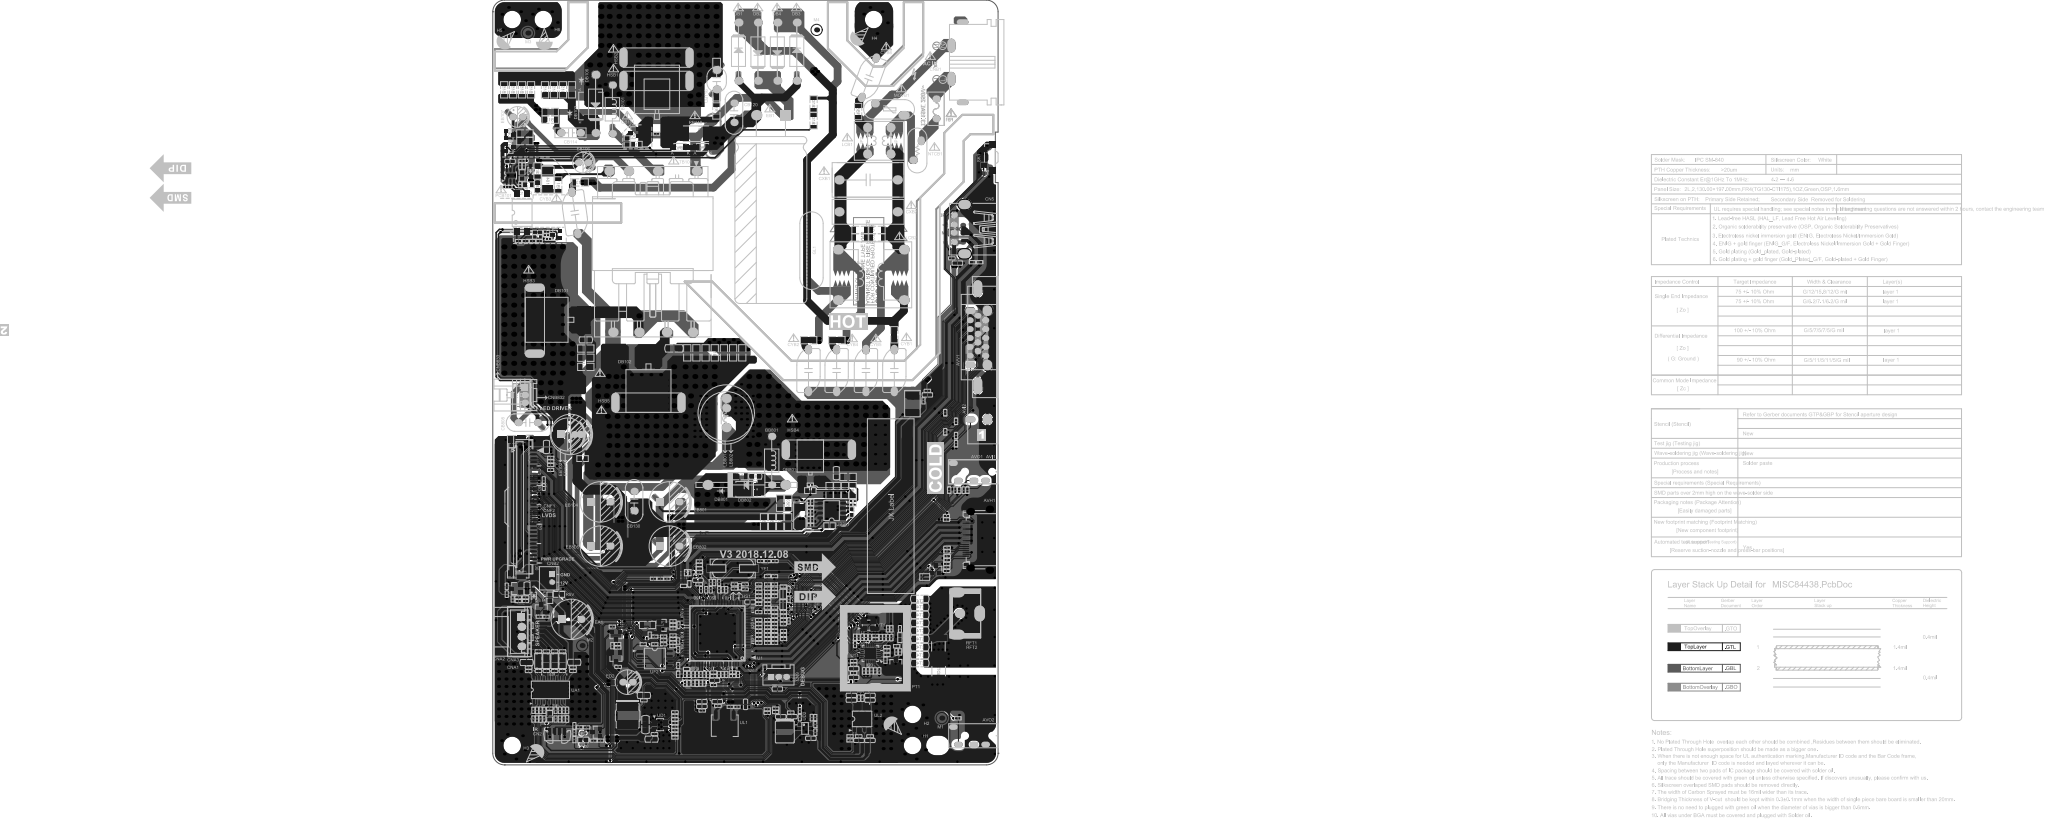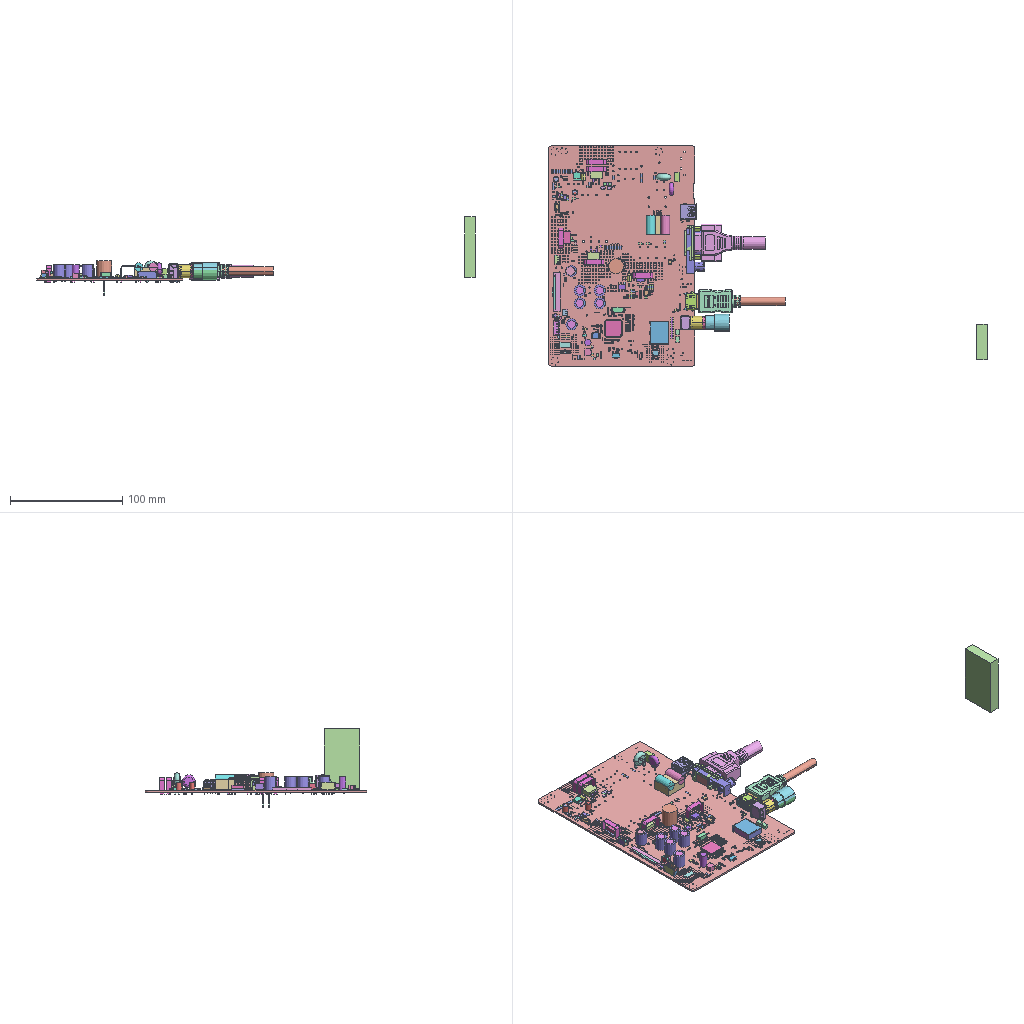Circuit board layout | Altium Designer | box 390.7 x 197 x 69.7 mm
Layer stack:
# Altium Designer layer stack of  (unit mm; dielectric type: 0 none, 1 core, 2 prepreg, 3 surface material)
index,name,kind,layer,copper_thickness_mm,dielectric_type,dielectric_thickness_mm,dielectric_material,dielectric_constant
0,TopPaste,other,,,,,,
1,TopOverlay,other,,,,,,
2,TopSolder,dielectric,,,3,0.0102,Solder Resist,3.5
3,TopLayer,copper,TopLayer,0.0356,,,,
4,Dielectric1,dielectric,,,1,1.5,FR-4,4.8
5,BottomLayer,copper,BottomLayer,0.0356,,,,
6,BottomSolder,dielectric,,,3,0.0102,Solder Resist,3.5
7,BottomOverlay,other,,,,,,
8,BottomPaste,other,,,,,,
# drill layer pairs: low layer,high layer
drill_pair,TopLayer,BottomLayer
Part placement, first 381 of 575 lines:
Designator,Comment,Layer,Footprint,Center-X(mm),Center-Y(mm),Rotation
CYB6,Y capacitor,CAP Y1,CD,100pF,400VAC,±10%,KS,10mm,Y5P,DIP,Walsin,TopLayer,CAP13*5-V-10-1,-33.2,177,70
CB116,Ceramic capacitor,CAP CD,2KV,68pF,±5%,SL,IK,5.0mm,DIP,TP,Walsin,TopLayer,CAP6.5*5-V-5-1,-72.401,176.521,90
CB120,Ceramic capacitor,CAP CD,2KV,4700pF,±20%,Y5U,IK,5.0mm,DIP,TP,Walsin,TopLayer,CAP10*4.5-V-5,-67.939,167.989,90
RB119,Thick-film resistor,RES,1/4W,10ohm,±5%,1206,SMD,TopLayer,R1206,-72.477,168.453,90
CNF1,NC/FFC socket,FFC connector,30Pin,D1.0,Bottom,lock,SMD,F10033FA030M1WL,CT,TopLayer,FFC30H/1.0S-7,-122.333,66.5,270
CAUTION,CAUTION,BottomLayer,CAUTION,-684.727,-474.313,90
TB-GND2,NC/TEST,BottomLayer,TP-10,-35.979,193.624,90
TB-GND1,NC/TEST,BottomLayer,TP-10,-119.545,188.239,90
H6,Location hole,TopLayer,ASSE4.0C-3,-116.613,191.96,0
H5,Location hole,TopLayer,ASSE4.0C-3,-124.715,191.746,0
HOT,HOT,TopLayer,HOT,-684.727,-474.313,360
High Voltage,High Voltage,TopLayer,High_Voltage,-684.727,-474.313,360
H4,Location hole,TopLayer,ASSE4.0C-3,-31.653,191.758,0
COLD,COLD,TopLayer,COLD,-684.727,-474.313,90
M3,MARK,TopLayer,MARK,-120.968,188.519,0
M4,MARK,TopLayer,MARK,-46.685,189.332,0
RB106,Thick-film resistor,RES,1/8W,68ohm,±5%,0805,SMD,TopLayer,R0805,-93.04,159.88,360
CB801,Ceramic capacitor,CAP MC,25V,1uF,±10%,X7R,0603,SMD,TP,TopLayer,C0603,-37.668,65.113,270
RB816,10ohm-0805-±5%-1/8W,TopLayer,R0805,-43.355,61.595,360
BB101,Ferrite bead,BEAD,70ohmMin,f3.5×6.0×0.65,DIP,TP,RH3.5×6×0.8-T-LF,DL,TopLayer,LB/3.5*6*12.5,-99.228,168.874,270
DB106,Rectifier diode,DIO FRD S,2A,1000V,DO-15,DIP,FR207G-FG-WS,WILLAS,TopLayer,D2-H-15,-103.554,170.282,270
CXB1,X capacitor,CAP X2,MP,275VAC,0.47uF,±10%,S,15mm-Mini,PC,DIP,BM,TopLayer,CAP18*8.5-V-15,-33.432,150.692,180
JP2,NC/Jumper,RES JUMP,0.6,7.0mm,DIP,TopLayer,JP7.0,-33.582,160.763,90
JP1,NC/Jumper,RES JUMP,0.6,7.0mm,DIP,TopLayer,JP7.0,-27.582,160.763,90
NTCB1,SCK102R55AMBY502 (short leg / Weiqin),TopLayer,NTC(10*5)-V5,-20.812,158.268,90
TB101,Transformer,EQ2914,310uH,0.30×2P,29Ts,H14.5MAX,SYEQ2914Z-T012021A (BLACK),DIP,YX,TopLayer,T/EQ2914*9-1,-88.835,132.192,270
LB802,NC/Differential-mode inductor,Inductor,DR12×14,68uH,0.45,20Ts,H13.5MAX,SYDR1214-L068uA,DIP,Soldier,TopLayer,L(13.5*15.5)-V-5,-69.945,89.4,90
RB835,Thick-film resistor,RES,1/4W,270Kohm,±1%,1206-Auto,SMD,TopLayer,R1206,-53.993,67.399,90
LCB2,Common-mode choke,Common Choke,UC1614,10.5mH±10%,0.15×1.0mm,48Ts,H14.0MAX,SYUC16-L10.5mA,DIP,CH,TopLayer,L/LC4/21*17-H-17*13,-32.722,126.231,180
BB801,Ferrite bead,BEAD,30ohmMin,F3.5×3.0×0.65,DIP,TP,RH3.5×3×0.8-T-LF,DL,TopLayer,LB/3.5*6*12.5,-58.242,78.364,270
CB101,100pF-0402-NPO-±5%-50V,TopLayer,C0402,-122.936,154.254,270
CB102,0.1uF-0603-X7R-±10%-50V,TopLayer,C0603,-125.565,155.473,180
CB103,Ceramic capacitor,CAP MC,50V,1000pF,±20%,X7R,0402,SMD,TP,TopLayer,C0402,-125.882,148.882,180
CB109,Ceramic capacitor,CAP MC,25V,0.22uF,±10%,X7R,0603,SMD,TP,TopLayer,C0603,-118.504,137.198,360
CB110,NC/1000pF-0402-X7R-±10%-50V,TopLayer,C0402,-116.205,137.351,360
CB113,NC/220PF-0805-NPO-±10%-200V,TopLayer,C0805,-118.478,149.022,90
CB114,Film capacitor,CAP PE,400V,4700pF,±5%,P,5.0mm,PC,DIP,TP,Fara,TopLayer,CAP8*2.5-V-5,-110.007,162.814,360
CB117,1000pF-0805-NPO-±10%-200V,TopLayer,C0805,-106.07,109.479,360
CB118,Ceramic capacitor,CAP MC,1KV,1000pF,±5%,NPO,1206,SMD,TP,TopLayer,C1206,-83.384,107.288,360
CB125,NC/Ceramic capacitor,CAP MC,50V,0.022uF,±10%,X7R,0402,SMD,TP,TopLayer,C0402,-121.59,134.925,360
CB130,Ceramic capacitor,CAP CD,1KV,4700pF,±20%,Y5U,IK,5.0mm,DIP,TP,Walsin,TopLayer,CAP10*4.5-V-5,-93.638,67.958,90
CB803,100pF-0402-NPO-±5%-50V,TopLayer,C0402,-37.821,67.496,90
CB804,4700pF-0402-X7R-±10%-50V,TopLayer,C0402,-47.803,67.653,90
CB805,NC/0.1uF-0402-X7R-±10%-16V,TopLayer,C0402,-48.73,64.91,90
CB806,Ceramic capacitor,CAP MC,50V,1000pF,±20%,X7R,0402,SMD,TP,TopLayer,C0402,-47.803,63.132,270
CB808,NC/Ceramic capacitor,CAP CD,1KV,4700pF,±20%,Y5U,K,5.0mm,DIP,TP,Walsin,TopLayer,CAP10*4.5-V-5,-120.983,88.168,180
CB809,Ceramic capacitor,CAP MC,500V,220pF,±5%,NPO,0805,SMD,TP,TopLayer,C0805,-41.618,75.146,90
CB810,Ceramic capacitor,CAP MC,500V,220pF,±5%,NPO,0805,SMD,TP,TopLayer,C0805,-62.466,74.364,180
CB812,0.033uF-0402-X7R-±10%-16V,TopLayer,C0402,-47.803,64.91,90
CB813,100pF-0402-NPO-±5%-50V,TopLayer,C0402,-47.803,61.366,90
CNB1,Red-phosphorus-free connector socket,connect jack(HP),2Pin,D8.6,L,SNAP,Fool-proofing,Black,L=4.0mm,DIP,YQ,TopLayer,CON2-H8.6-1,-9.9,181,90
CNB832,NC/Connector socket,connect jack,3Pin,D2.0,D,SNAP,L=2.8mm,DIP,CNJST,TopLayer,SIP3/2.0D-CP,-121.744,95.263,270
Conformal Coating,NC/Conformal coating,25kg/Can,Peters,TopLayer,Conformal_Coating,-147.574,131.394,90
CXB2,NC/X capacitor,CAP X2,MP,280VAC,0.1uF,±10%,P,15mm,PC,DIP,JH,TopLayer,CAP18*5*11.5-V-15,-33.432,142.471,360
CYB2,Y capacitor,CAP Y1,CD,470pF,400VAC,±20%,KS,10mm,Y5U,DIP,Walsin,TopLayer,CAP13*5-V-10-1,-48.777,101.582,270
CYB3,Y capacitor,CAP Y1,CD,470pF,400VAC,±20%,KS,10mm,Y5U,DIP,Walsin,TopLayer,CAP13*5-V-10-1,-108.882,142.227,278
CYB4,NC/Y capacitor,CAP Y1,CD,47pF,400VAC,±5%,KS,10mm,SL,DIP,BULK,Walsin,TopLayer,CAP13*5-V-10-1,-41.538,101.582,270
CYB5,NC/Y capacitor,CAP Y1,CD,47pF,400VAC,±5%,KS,10mm,SL,DIP,BULK,Walsin,TopLayer,CAP13*5-V-10-1,-33.994,101.582,270
DB1,Rectifier diode,DIO SI S,2.5A,1000V,DO-15,DIP,RL257G,YJ,TopLayer,D2-H-15,-66.788,183.722,90
DB2,Rectifier diode,DIO SI S,2.5A,1000V,DO-15,DIP,RL257G,YJ,TopLayer,D2-H-15,-61.788,183.722,270
DB3,Rectifier diode,DIO SI S,2.5A,1000V,DO-15,DIP,RL257G,YJ,TopLayer,D2-H-15,-51.788,183.722,90
DB4,Rectifier diode,DIO SI S,2.5A,1000V,DO-15,DIP,RL257G,YJ,TopLayer,D2-H-15,-56.788,183.722,270
DB101,Schottky diode,DIO SBD D1,10A,150V,TO-263,SMD,HBR10150SS,JLHW,TopLayer,D2PAK3,-111.791,114.655,90
DB102,Schottky diode,DIO SBD D1,10A,200V,TO-263,SMD,HBR10200SS,JLHW,TopLayer,D2PAK3,-89.948,100.645,180
DB103,NC/Rectifier diode,DIO SI S,3A,1000V,SMC,SMD,HS3M R6,TSC,TopLayer,DIODE-SMC,-104.775,169.723,90
DB104,Rectifier diode,DIO SI S,1A,1000V,SMAF,SMD,M7F,YJ,TopLayer,DIODE-S-2,-115.83,150.795,90
DB109,Rectifier diode,DIO FRD S,1.2A,800V,SOD-123FL,SMD,F1K,YJ,TopLayer,DIODE-S-14,-81.842,159.075,180
DB110,Rectifier diode,DIO FRD S,1.2A,800V,SOD-123FL,SMD,F1K,YJ,TopLayer,DIODE-S-14,-76.028,159.075,180
DB111,Switching diode,DIO SW D1,215mA,85V,SOT-23,SMD,KAV70,KEXIN,TopLayer,SO-23,-93.612,162.839,270
DB112,NC/Switching diode,DIO SW S,200mA,250V,SOD-323,SMD,BAV21WS,BLUE ROCKET,TopLayer,DIODE-S-12,-120.307,152.971,270
DB801,Schottky diode,DIO SBD S,3A,100V,DO-201AD,DIP,SR3100,YJ,TopLayer,D3-H-20-2,-64.742,72.114,180
DB802,NC/TSPB5H150S,TopLayer,DIODE-S-13,-63.971,70.989,90
DB804,Rectifier diode,DIO SI S,1A,1000V,SMAF,SMD,M7F,YJ,TopLayer,DIODE-S-2,-50.99,64.224,270
EB1,Aluminum electrolytic capacitor,CAP AL,450V,82uF,±20%,SL,KL,BK,7.5mm,18×35.5,DIP,CapXon,TopLayer,EC(18*41)-H-7.5-1,-58.458,167.359,360
EB101,Aluminum electrolytic capacitor,CAP AL,25V,470uF,±20%,LD,GK,P,5.0mm,10×12.5,DIP,TP,Samxon,TopLayer,EC(10*12.5)-V-5,-110,84.288,360
EB102,NC/270uF-16V-±20%-8×11-105℃-RP-short leg-F=3.5(Elite),TopLayer,EC(8*11)-V-3.5,-110.75,85.114,360
EB104,Aluminum electrolytic capacitor,CAP AL,63V,100uF,±20%,LD,GF,P,5.0mm,10×12.5,DIP,TP,CapXon,TopLayer,EC(10*12.5)-V-5,-99.904,67.951,360
EB105,Aluminum electrolytic capacitor,CAP AL,63V,100uF,±20%,LD,GF,P,5.0mm,10×12.5,DIP,TP,CapXon,TopLayer,EC(10*12.5)-V-5,-102.311,55.624,360
EB106,Aluminum electrolytic capacitor,CAP AL,50V,10uF,±20%,LF,GH,P,2.5mm,5×11,DIP,TP,CapXon,TopLayer,EC(5*11)-V-2.5,-106.782,154.745,360
EB107,NC/Aluminum electrolytic capacitor,CAP AL,50V,4.7uF,±20%,LC,LL,P,2.5mm,5×11,DIP,TP,CapXon,TopLayer,EC(5*11)-V-2.5,-123.652,166.523,360
EB801,Aluminum electrolytic capacitor,CAP AL,100V,47uF,±20%,LD,SF,P,5.0mm,10×12.5,DIP,TP,Samxon,TopLayer,EC(10*12.5)-V-5,-84.573,66.967,360
EB802,NC/47uF-100V-±20%-10×12-105℃-EV-taped reel-F=5.0(Elite),TopLayer,EC(10*12.5)-V-5,-84.573,55.36,360
FB1,Slow-blow fuse,FUSE T,P,3.15A,250VAC,8.5×4.0×8mm,DIP,TP,Walter,TopLayer,FUSE8.5*4-V-5(T3.15AL_250V~),-15.953,169.012,90
GL1,Silicone,0.5g,general,60,white,SLD-8854W,XY,TopLayer,Silica_gel-20,-684.727,-474.313,180
HSB1,NC/17.5×14.5×0.5- natural finish -Cu-MRD,TopLayer,HS038,-87.874,176.188,180
HSB2,NC/17.5×14.5×0.5- natural finish -Cu-MRD,TopLayer,HS038,-87.874,182.188,180
HSB3,NC/17.5×14.5×0.5- natural finish -Cu-MRD,TopLayer,HS038,-119.2,114.438,270
HSB4,NC/17.5×14.5×0.5- natural finish -Cu-MRD,TopLayer,HS038,-46.126,81.193,360
HSB5,NC/17.5×14.5×0.5- natural finish -Cu-MRD,TopLayer,HS038,-89.948,93.305,180
LB801,Differential-mode inductor,Inductor,DR12×12,70uH,0.15×12P,38.5Ts,H13.5MAX,SYDR1212-L070uA,DIP,DL,TopLayer,L/LC2/15*14.5-V7.5,-69.945,90.65,90
LCB1,Common-mode choke,Common Choke,T9×5×3,230uH MIN,0.45×1P,7.5Ts,H14.0MAX,SYT09-L230uA,DIP,CK,TopLayer,L/LC4/12.8*10-V-6*7,-30.582,160.763,180
MOVB1,Varistor,VARISTOR,128J,680V,4000A,S,7.5mm,10mm,DIP,Thinking,TopLayer,VR(13*5)-V-7.5,-27.932,168.866,360
PCB101,LTV-817S-TA-B (Lite-On),TopLayer,OC4-S-1,-122.45,142.227,360
QB801,MOSFET,NMOS,15A,100V,0.105ohm@ID=6A@VGS=10V,TO-252,PA110BDA,UNIKC,TopLayer,TO-252-GDS,-48.311,76.715,360
RB1,1M2ohm-1206-±5%-1/4W,TopLayer,R1206,-31.168,137.812,180
RB2,1M2ohm-1206-±5%-1/4W,TopLayer,R1206,-31.168,135.851,180
RB3,1M2ohm-1206-±5%-1/4W,TopLayer,R1206,-35.511,137.811,180
RB4,1M2ohm-1206-±5%-1/4W,TopLayer,R1206,-35.511,135.849,180
RB5,NC/0ohm-1206-PCB-D,TopLayer,R1206SC,-41.47,109.398,180
RB6,NC/0ohm-1206-PCB-D,TopLayer,R1206SC,-26.7,110.8,270
RB7,NC/0ohm-1206-PCB-D,TopLayer,R1206SC,-48.734,109.398,180
RB101,330Kohm-1206-±5%-1/4W,TopLayer,R1206,-47.473,170.256,270
RB102,330Kohm-1206-±5%-1/4W,TopLayer,R1206,-47.473,165.938,270
RB103,Thick-film resistor,RES,1/16W,3.6Kohm,±1%,0402,SMD,TopLayer,R0402,-122.022,154.254,90
RB104,Thick-film resistor,RES,1/16W,39Kohm,±1%,0402,SMD,TopLayer,R0402,-122.936,149.428,270
RB105,Thick-film resistor,RES,1/16W,510ohm,±1%,0402,SMD,TopLayer,R0402,-122.479,155.613,360
RB107,Thick-film resistor,RES,1/8W,20ohm,±5%,0805,SMD,TopLayer,R0805,-95.462,160.596,90
RB109,Thick-film resistor,RES,1/16W,10Kohm,±1%,0402,SMD,TopLayer,R0402,-87.871,162.598,180
RB110,0ohm-1206-±5%-1/4W,TopLayer,R1206,-121.742,160.68,360
RB111,0ohm-1206-±5%-1/4W,TopLayer,R1206,-121.742,162.655,360
RB112,NC/33Kohm-0805-±1%-1/8W,TopLayer,R0805,-122.479,151.816,270
RB113,Thick-film resistor,RES,1/8W,300Kohm,±1%,0805,SMD,TopLayer,R0805,-120.879,149.428,360
RB114,Thick-film resistor,RES,1/4W,4.7ohm,±1%,1206,SMD,TopLayer,R1206,-113.16,149.395,90
RB116,NC/10ohm-1206-±5%-1/4W,TopLayer,R1206,-118.478,152.984,90
RB117,Thick-film resistor,RES,1/4W,10ohm,±5%,1206,SMD,TopLayer,R1206,-115.222,166.201,180
RB118,Thick-film resistor,RES,1/4W,10ohm,±5%,1206,SMD,TopLayer,R1206,-115.222,168.205,180
RB124,68ohm-1206-±5%-1/4W,TopLayer,R1206,-65.813,106.142,270
RB125,68ohm-1206-±5%-1/4W,TopLayer,R1206,-70.533,106.142,270
RB126,68ohm-1206-±5%-1/4W,TopLayer,R1206,-75.253,106.142,270
RB127,68ohm-1206-±5%-1/4W,TopLayer,R1206,-79.973,106.142,270
RB128,Thick-film resistor,RES,1/4W,47ohm,±5%,1206,SMD,TopLayer,R1206,-106.07,107.241,180
RB129,Thick-film resistor,RES,1/4W,47ohm,±5%,1206,SMD,TopLayer,R1206,-106.07,102.521,180
RB130,30ohm-1206-±5%-1/4W,TopLayer,R1206,-107.507,150.028,180
RB131,Thick-film resistor,RES,1/10W,2Kohm,±5%,0603,SMD,TopLayer,R0603,-118.504,135.992,360
RB132,Thick-film resistor,RES,1/16W,1.2Kohm,±1%,0402,SMD,TopLayer,R0402,-123.393,134.929,180
RB133,Thick-film resistor,RES,1/16W,10Kohm,±1%,0402,SMD,TopLayer,R0402,-116.205,136.423,180
RB134,Thick-film resistor,RES,1/16W,4.7Kohm,±1%,0402,SMD,TopLayer,R0402,-115.7,135.5,180
RB135,Thick-film resistor,RES,1/16W,18Kohm,±1%,0402,SMD,TopLayer,R0402,-118.054,134.925,360
RB140,Thick-film resistor,RES,1/8W,51Kohm,±1%,0805,SMD,TopLayer,R0805,-106.9,78.9,180
RB148,Thick-film resistor,RES,2W,0.22ohm,±5%,2512,SMD,TopLayer,R2512-1,-77.737,162.59,180
RB150,150Kohm-1206-±5%-1/4W,TopLayer,R1206,-124.769,173.897,270
RB151,150Kohm-1206-±5%-1/4W,TopLayer,R1206,-122.469,173.897,270
RB152,150Kohm-1206-±5%-1/4W,TopLayer,R1206,-127.07,173.897,270
RB153,150Kohm-1206-±5%-1/4W,TopLayer,R1206,-114.266,173.897,90
RB155,150Kohm-1206-±5%-1/4W,TopLayer,R1206,-111.966,173.897,90
RB156,NC/150Kohm-1206-±5%-1/4W,TopLayer,R1206,-120.168,173.897,270
RB157,NC/150Kohm-1206-±5%-1/4W,TopLayer,R1206,-116.567,173.897,90
RB158,NC/Thick-film resistor,RES,1/16W,51ohm,±1%,0402,SMD,TopLayer,R0402,-119.781,134.925,360
RB162,NC/68ohm-1206-±5%-1/4W,TopLayer,R1206,-68.173,106.142,270
RB163,NC/68ohm-1206-±5%-1/4W,TopLayer,R1206,-72.893,106.142,270
RB164,NC/68ohm-1206-±5%-1/4W,TopLayer,R1206,-77.613,106.142,270
RB165,NC/68ohm-1206-±5%-1/4W,TopLayer,R1206,-106.07,104.881,180
RB803,Thick-film resistor,RES,1/16W,18Kohm,±1%,0402,SMD,TopLayer,R0402,-48.73,63.132,90
RB804,NC/10Kohm-0402-±5%-1/16W,TopLayer,R0402,-48.26,66.294,360
RB805,100ohm-0402-±5%-1/16W,TopLayer,R0402,-48.73,67.666,90
RB806,Thick-film resistor,RES,1/16W,1Kohm,±1%,0402,SMD,TopLayer,R0402,-36.893,67.496,90
RB807,20ohm-0805-±5%-1/8W,TopLayer,R0805,-48.311,70.65,180
RB808,10Kohm-0402-±1%-1/16W,TopLayer,R0402,-48.311,72.2,180
RB810,Thick-film resistor,RES,1/4W,10ohm,±5%,1206,SMD,TopLayer,R1206,-38.593,74.18,360
RB812,Thick-film resistor,RES,1/4W,10ohm,±5%,1206,SMD,TopLayer,R1206,-66.416,74.364,180
RB813,100ohm-0402-±5%-1/16W,TopLayer,R0402,-48.73,61.366,270
RB814,Thick-film resistor,RES,1/4W,270Kohm,±1%,1206-Auto,SMD,TopLayer,R1206,-56.069,67.399,270
RB818,Thick-film resistor,RES,1/4W,0.2ohm,±1%,1206,SMD,TopLayer,R1206,-37.423,70.65,270
RB819,Thick-film resistor,RES,1/4W,0.2ohm,±1%,1206,SMD,TopLayer,R1206,-39.404,70.65,270
RB820,Thick-film resistor,RES,1/4W,0.2ohm,±1%,1206,SMD,TopLayer,R1206,-41.386,70.65,270
RB821,Thick-film resistor,RES,1/4W,0.2ohm,±1%,1206,SMD,TopLayer,R1206,-43.354,70.65,270
RB837,Thick-film resistor,RES,1/4W,1.5ohm,±1%,1206,SMD,TopLayer,R1206,-60.221,62.611,90
RB838,Thick-film resistor,RES,1/4W,1.6ohm,±1%,1206,SMD,TopLayer,R1206,-58.145,62.611,90
RB839,Thick-film resistor,RES,1/4W,3.3ohm,±1%,1206,SMD,TopLayer,R1206,-56.069,62.611,270
RB840,NC/1R5ohm-1206-±1%-1/4W,TopLayer,R1206,-53.993,62.611,90
TP-TDT,NC/,BottomLayer,TP-TDT,-73.368,161.976,270
UB101,PWM controller,IC PWM Controller,100KHz,SOT23-6,SMD,LD5523B GL,Leadtrend,TopLayer,SOT-26,-125.45,151.827,180
UB102,AZ431AN-ATRE1(BCD),TopLayer,SOT-23-RAK,-113.666,136.612,90
UB801,PWM controller,IC PWM Controller,120KHz,SOP-8,SMD,OB3353ACPA,ON-Bright,TopLayer,SO-8A,-42.824,65.507,180
ZDB1,NC/BZX84C24 (Blue Rocket),TopLayer,SO-23,-125.679,159.093,90
ZDB2,NC/Switching diode,DIO SW D1,215mA,85V,SOT-23,SMD,KAV70,KEXIN,TopLayer,SO-23,-125.679,162.369,90
RB154,150Kohm-1206-±5%-1/4W,TopLayer,R1206,-109.665,173.897,90
CYB1,Y capacitor,CAP Y1,CD,470pF,400VAC,±20%,KS,10mm,Y5U,DIP,Walsin,TopLayer,CAP13*5-V-10-1,-26.691,101.582,270
QB101,MOSFET,NMOS,7A,650V,0.55ohm@ID=3.5A@VGS=10V,TO-252,LSG65R650HT,LONTEN,TopLayer,D2PAK3,-87.771,169.051,270
PWM_REF,NC/TEST,BottomLayer,TP_BL,-97.663,46.99,90
CNB2,Connector socket,connect jack,2Pin,D2.0,D,Beige,L=2.8mm,DIP,W2011-02SVA-SN8-ENSY,XYDT,TopLayer,SIP2/2.0D-1,-114.808,48.057,270
DU2,NC/,TopLayer,DIODE-S0402,-79.426,46.66,270
DU1,NC/,TopLayer,DIODE-S0402,-80.899,46.101,360
CU4,NC/10uF-0603-X5R-±20%-6.3V,TopLayer,C0603,-18.186,95.301,180
CU3,NC/Ceramic capacitor,CAP MC,6.3V,0.47uF,±10%,X5R,0402,SMD,TP,TopLayer,C0402,-18.186,96.368,360
AI_V,AI_GRIPPER_V,TopLayer,AI_GRIPPER_V,256.019,35.242,90
LD3,Power inductor,Power Inductor,4.7uH,±20%,2.8A,0.32×1P,DR5.8×4.5,SMD,PIO54-4R7MTP02,FH,TopLayer,L(6.0*4.5)-S,-95.301,12.649,90
RL5,91ohm-0402-±1%-1/16W,TopLayer,R0402,-38.087,6.299,360
RL4,150ohm-0402-±1%-1/16W,TopLayer,R0402,-38.087,7.367,0
1.8V_DDR,TEST,BottomLayer,TP,-74.587,20.066,180
NO DOLBY,NO DOLBY,BottomLayer,NO_DOLBY-SILK,-684.727,-474.313,360
CNA2,Connector socket,connect jack,4PIN,D2.50,L,SNAP,STEP,Fool-proofing,Nature,L=3.0mm,DIP,AMA,TopLayer,SIP4H/2.54D-2,-122.636,34.29,270
S/N2,Barcode,BottomLayer,Barcode,-57.912,47.879,0
XXXXXXXXXXXXXXX,PCB_NAME,TopLayer,PCB_NAME,-67.793,58.272,90
Manufacture_Info,Manufacture_Info,TopLayer,Manufacture_Info,-73.4,33.6,180
M2,MARK,TopLayer,MARK,-107.01,30.734,0
M1,MARK,TopLayer,MARK,-14.478,12.052,0
CQC,CQC,TopLayer,CQC,-684.727,-474.313,270
S/N1,Barcode,BottomLayer,Barcode,-29.8,74.6,270
XXXXXX,PCB_TIME,TopLayer,PCB_TIME,-71.756,61.053,90
3V3_TU,TEST,BottomLayer,TP,-38.557,20.498,270
1.15V_STB,TEST,BottomLayer,TP,-68.567,17.551,270
3V3_STB,TEST,BottomLayer,TP,-68.567,22.123,90
5V_STB,TEST,BottomLayer,TP,-99.085,21.234,0
AVH1,HDMI terminal,HDMI Jack,H,Block up,SMD,51U019S-313HFN-E-R-F,FREEPORT,TopLayer,HDMI-HS-11,-5.25,58,90
AVI1,NC/Earphone terminal,Earphone Jack,H,F3.6,CH5.5,Black,Seal,DIP,PJ-320B-F5.5,JSL,TopLayer,PHONE-HD-43,-6.522,75.5,90
AVO1,Earphone terminal,Earphone Jack,H,F3.6,CH5.5,Black,Seal,DIP,PJ-320B-F5.5,JSL,TopLayer,PHONE-HD-43,-6.522,75.5,90
AVO2,NC/Earphone terminal,Earphone Jack,H,F3.6,CH5.5,Black,Seal,DIP,PJ-320B-F5.5,JSL,TopLayer,PHONE-HD-43,-6.5,7.5,90
AVV1,NC/WLHD-051A,TopLayer,DB15-HF-1,-5.247,110.2,90
CD1,10uF-0805-X5R-±20%-16V,TopLayer,C0805,-89.154,6.629,360
CD2,0.1uF-0402-X5R-±20%-16V,TopLayer,C0402,-83.146,13.551,360
CD11,10uF-0603-X5R-±20%-6.3V,TopLayer,C0603,-48.171,6.858,360
CD12,NC/0.1uF-0402-X5R-±20%-16V,TopLayer,C0402,-47.015,8.395,90
CD13,3300pF-0402-X7R-±10%-50V,TopLayer,C0402,-47.955,12.179,270
CD14,10uF-0603-X5R-±20%-6.3V,TopLayer,C0603,-53.027,12.421,180
CD15,10uF-0603-X5R-±20%-6.3V,TopLayer,C0603,-55.918,12.408,360
CD16,NC/0.1uF-0402-X5R-±20%-16V,TopLayer,C0402,-53.34,13.487,180
CD17,Ceramic capacitor,CAP MC,6.3V,1uF,±20%,X5R,0402,SMD,TP,TopLayer,C0402,-51.027,12.179,270
CD19,NC/0.1uF-0402-X5R-±20%-16V,TopLayer,C0402,-88.392,7.925,360
CD20,NC/22pF-0402-NPO-±5%-50V,TopLayer,C0402,-83.146,11.697,180
CD21,NC/0.1uF-0402-X5R-±20%-16V,TopLayer,C0402,-91.135,16.612,360
CD22,10uF-0805-X5R-±20%-16V,TopLayer,C0805,-91.123,17.894,360
CD41,NC/10uF-1206-X5R-±10%-16V,TopLayer,C1206,-90.715,10.377,270
CF1,33pF-0402-NPO-±5%-50V,TopLayer,C0402,-73.939,46.964,270
CF2,0.1uF-0402-X5R-±20%-16V,TopLayer,C0402,-86.055,31.064,360
CF4,33pF-0402-NPO-±5%-50V,TopLayer,C0402,-71.755,46.964,90
CF5,10uF-0603-X5R-±20%-6.3V,TopLayer,C0603,-56.794,19.558,360
CF7,0.1uF-0402-X5R-±20%-16V,TopLayer,C0402,-74.612,23.302,90
CF8,0.1uF-0402-X5R-±20%-16V,TopLayer,C0402,-61.57,31.445,180
CF9,0.1uF-0402-X5R-±20%-16V,TopLayer,C0402,-76.429,45.11,270
CF10,0.1uF-0402-X5R-±20%-16V,TopLayer,C0402,-61.57,36.347,180
CF12,0.1uF-0402-X5R-±20%-16V,TopLayer,C0402,-71.755,45.11,270
CF13,0.1uF-0402-X5R-±20%-16V,TopLayer,C0402,-61.57,39.344,180
CF14,0.1uF-0402-X5R-±20%-16V,TopLayer,C0402,-69.926,45.11,270
CF15,NC/10uF-0603-X5R-±20%-6.3V,TopLayer,C0603,-77.216,47.574,180
CF16,0.1uF-0402-X5R-±20%-16V,TopLayer,C0402,-76.911,46.507,360
CF17,0.1uF-0402-X5R-±20%-16V,TopLayer,C0402,-68.301,23.81,180
CF18,0.1uF-0402-X5R-±20%-16V,TopLayer,C0402,-78.435,23.314,90
CF19,0.1uF-0402-X5R-±20%-16V,TopLayer,C0402,-73.939,45.11,270
CF20,0.1uF-0402-X5R-±20%-16V,TopLayer,C0402,-82.296,29.705,90
CF21,0.1uF-0402-X5R-±20%-16V,TopLayer,C0402,-75.552,23.302,90
CF22,10uF-0603-X5R-±20%-6.3V,TopLayer,C0603,-72.936,21.79,360
CF23,Ceramic capacitor,CAP MC,6.3V,2.2uF,±20%,X5R,0402,SMD,TP,TopLayer,C0402,-75.082,45.11,270
CF24,0.1uF-0402-X5R-±20%-16V,TopLayer,C0402,-73.203,23.81,180
CF25,0.1uF-0402-X5R-±20%-16V,TopLayer,C0402,-73.203,22.872,180
CF26,0.047uF-0402-X7R-±10%-16V,TopLayer,C0402,-57.506,38.303,360
CF29,NC/1000pF-0402-X7R-±10%-50V,TopLayer,C0402,-57.233,14.516,360
CF30,NC/1000pF-0402-X7R-±10%-50V,TopLayer,C0402,-59.405,13.399,360
CF31,NC/0.047uF-0402-X7R-±10%-16V,TopLayer,C0402,-57.48,33.477,360
CF33,NC/5pF-0402-NPO-±5%-50V,TopLayer,C0402,-116.896,71.552,90
CF34,NC/0.047uF-0402-X7R-±10%-16V,TopLayer,C0402,-61.57,37.312,180
CF35,NC/5pF-0402-NPO-±5%-50V,TopLayer,C0402,-116.896,73.381,270
CF37,10uF-0603-X5R-±20%-6.3V,TopLayer,C0603,-64.973,15.596,270
CF38,NC/0.1uF-0402-X5R-±20%-16V,TopLayer,C0402,-126.416,43.98,270
CF39,NC/NC/30pF-0402-NPO-±5%-50V,TopLayer,C0402,-59.309,52.489,360
CF40,Ceramic capacitor,CAP MC,50V,1000pF,±20%,X7R,0402,SMD,TP,TopLayer,C0402,-57.429,52.489,180
CH8,NC/0.1uF-0402-X5R-±20%-16V,TopLayer,C0402,-13.183,51.791,360
CH9,NC/0.1uF-0402-X5R-±20%-16V,TopLayer,C0402,-13.208,49.962,360
CH10,NC/30pF-0402-NPO-±5%-50V,TopLayer,C0402,-13.132,55.956,180
CH15,NC/1uF-0402-X5R-±20%-16V,TopLayer,C0402,-68.301,22.872,180
CI1,NC/0.047uF-0402-X7R-±10%-16V,TopLayer,C0402,-59.309,36.347,360
CI3,NC/0.1uF-0402-X5R-±20%-16V,TopLayer,C0402,-61.57,42.431,360
CI4,NC/0.1uF-0402-X5R-±20%-16V,TopLayer,C0402,-59.309,42.431,360
CI6,0.1uF-0402-X5R-±20%-16V,TopLayer,C0402,-59.309,40.5,360
CI7,0.1uF-0402-X5R-±20%-16V,TopLayer,C0402,-59.309,41.452,360
CI8,0.047uF-0402-X7R-±10%-16V,TopLayer,C0402,-57.506,37.313,360
CK2,0.01uF-0402-X7R-±10%-50V,TopLayer,C0402,-77.483,23.302,270
CK4,0.1uF-0402-X5R-±20%-16V,TopLayer,C0402,-109.004,10.058,90
CK6,NC/10pF-0402-NPO-±5%-50V,TopLayer,C0402,-83.642,31.496,360
CK10,NC/0.1uF-0402-X5R-±20%-16V,TopLayer,C0402,-105.867,9.652,180
CL1,NC/10uF-0603-X5R-±20%-6.3V,TopLayer,C0603,-72.238,16.281,360
CL2,0.1uF-0402-X5R-±20%-16V,TopLayer,C0402,-72.085,15.215,360
CL6,0.1uF-0402-X5R-±20%-16V,TopLayer,C0402,-35.852,7.366,360
CL3,Ceramic capacitor,CAP MC,6.3V,1uF,±20%,X5R,0402,SMD,TP,TopLayer,C0402,-76.117,14.002,360
CL4,NC/10uF-0603-X5R-±20%-6.3V,TopLayer,C0603,-76.203,16.281,360
CL5,NC/10uF-0603-X5R-±20%-6.3V,TopLayer,C0603,-76.203,15.07,360
CL10,NC/0.1uF-0402-X5R-±20%-16V,TopLayer,C0402,-35.827,17.17,270
CL12,NC/10uF-0603-X5R-±20%-6.3V,TopLayer,C0603,-37.744,16.688,180
CL13,NC/0.1uF-0402-X5R-±20%-16V,TopLayer,C0402,-34.887,17.17,90
CM1,0.22uF-0402-X5R-±10%-16V,TopLayer,C0402,-97.866,30.233,360
CM2,0.1uF-0402-X5R-±20%-16V,TopLayer,C0402,-97.765,25.248,180
CM3,NC/0.1uF-0402-X5R-±20%-16V,TopLayer,C0402,-121.577,43.142,360
CM4,0.1uF-0402-X5R-±20%-16V,TopLayer,C0402,-126.416,45.987,90
CM5,NC/10uF-0805-X5R-±20%-16V,TopLayer,C0805,-121.196,45.428,90
CM7,0.022uF-0402-X7R-±10%-16V,TopLayer,C0402,-123.457,43.142,180
CN2,IR receiver transistor,IR Receriver,2.7-5.5V,37.9KHz,SMD,SIRAB39,SL,TopLayer,REMOTE-HS-1,-113.4,8.502,0
CN5,USB terminal,USB Jack,USB2.0,H,Single,Black,flange,Block up,DIP,103411481,VAST,TopLayer,USB-HD-30,-9.96,138,90
CN9,NC/Connector socket,connect jack,3Pin,D2.0,D,SNAP,Nature,L=2.8mm,DIP,AMA,TopLayer,SIP3/2.0D-3,-56.5,22.687,360
CNF2,FFC socket,FFC connector,30Pin,D1.0,Bottom,SMD,P-TWO,TopLayer,FFC30H/1.0S-1,-121.111,66.5,270
CO1,1uF-0402-X5R-±20%-6.3V,TopLayer,C0402,-57.506,44.475,360
CO3,NC/1000pF-0402-X7R-±10%-50V,TopLayer,C0402,-61.57,43.459,180
CO4,1uF-0402-X5R-±20%-6.3V,TopLayer,C0402,-59.309,45.415,180
CO5,NC/1000pF-0402-X7R-±10%-50V,TopLayer,C0402,-61.57,44.475,180
CO9,100pF-0402-NPO-±5%-50V,TopLayer,C0402,-57.506,39.344,180
CT1,0.1uF-0402-X5R-±20%-16V,TopLayer,C0402,-36.805,31.013,90
CT3,NC/10uF-0603-X5R-±20%-6.3V,TopLayer,C0603,-37.16,22.543,360
CT5,0.1uF-0402-X5R-±20%-16V,TopLayer,C0402,-37.16,25.845,360
CT6,10uF-0603-X5R-±20%-6.3V,TopLayer,C0603,-37.16,24.765,180
CT7,33pF-0402-NPO-±5%-50V,TopLayer,C0402,-28.346,32.791,270
CT8,33pF-0402-NPO-±5%-50V,TopLayer,C0402,-27.432,32.791,270
CT9,0.1uF-0402-X5R-±20%-16V,TopLayer,C0402,-30.544,24.206,270
CT10,33pF-0402-NPO-±5%-50V,TopLayer,C0402,-65.107,45.212,360
CT11,0.022uF-0402-X7R-±10%-16V,TopLayer,C0402,-33.533,24.206,90
CT12,0.022uF-0402-X7R-±10%-16V,TopLayer,C0402,-34.461,24.206,270
CT13,NC/1.2pF-0402-NPO-±0.25pf-50V,TopLayer,C0402,-26.167,29.103,270
CT17,NC/180pF-0402-NPO-±5%-50V,TopLayer,C0402,-25.248,35.039,90
CT18,0.1uF-0402-X5R-±20%-16V,TopLayer,C0402,-37.16,26.772,360
CT19,0.022uF-0402-X7R-±10%-16V,TopLayer,C0402,-61.57,46.507,180
CT20,0.1uF-0402-X5R-±20%-16V,TopLayer,C0402,-67.825,45.415,180
CT21,0.047uF-0402-X7R-±10%-16V,TopLayer,C0402,-28.613,30.39,360
CT23,0.1uF-0402-X5R-±20%-16V,TopLayer,C0402,-67.825,46.507,180
CT24,33pF-0402-NPO-±5%-50V,TopLayer,C0402,-65.107,46.507,180
CT25,0.1uF-0402-X5R-±20%-16V,TopLayer,C0402,-29.273,32.791,90
CT26,330pF-0402-NPO-±5%-50V,TopLayer,C0402,-31.572,32.346,360
CT27,0.1uF-0402-X5R-±20%-16V,TopLayer,C0402,-32.982,32.842,90
CT29,6800pF-0402-X7R-±10%-50V,TopLayer,C0402,-31.572,33.274,360
CT40,Ceramic capacitor,CAP MC,1KV,470pF,±5%,NPO,1206,SMD,TP,TopLayer,C1206,-20.142,32.449,180
CT41,4700pF-1206-X7R-±10%-1000V,TopLayer,C1206,-20.142,34.569,360
CT42,4700pF-1206-X7R-±10%-1000V,TopLayer,C1206,-20.142,30.328,360
CT43,4700pF-1206-X7R-±10%-1000V,TopLayer,C1206,-20.142,28.27,360
CT44,4700pF-1206-X7R-±10%-1000V,TopLayer,C1206,-20.142,36.601,360
CT45,4700pF-1206-X7R-±10%-1000V,TopLayer,C1206,-20.142,26.213,360
CT46,4700pF-1206-X7R-±10%-1000V,TopLayer,C1206,-20.142,38.633,360
CT47,NC/4700pF-1206-X7R-±10%-1000V,TopLayer,C1206,-20.142,42.746,360
CT48,4700pF-1206-X7R-±10%-1000V,TopLayer,C1206,-20.142,40.691,360
CU1,NC/10uF-0603-X5R-±20%-6.3V,TopLayer,C0603,-10.465,129.261,180
CU2,Ceramic capacitor,CAP MC,6.3V,0.47uF,±10%,X5R,0402,SMD,TP,TopLayer,C0402,-11.887,130.48,180
CV1,NC/0.047uF-0402-X7R-±10%-16V,TopLayer,C0402,-61.57,34.493,360
CV3,NC/0.047uF-0402-X7R-±10%-16V,TopLayer,C0402,-61.57,33.477,360
CV7,NC/0.047uF-0402-X7R-±10%-16V,TopLayer,C0402,-59.309,32.41,360
CV9,NC/33pF-0402-NPO-±5%-50V,TopLayer,C0402,-61.57,32.41,180
CV10,NC/33pF-0402-NPO-±5%-50V,TopLayer,C0402,-61.57,35.433,180
DH2,NC/0ohm-0402-±5%-1/16W,TopLayer,DIODE-S0402,-13.284,63.195,360
DH3,NC/NC/AVLC18S02003,TopLayer,DIODE-S0402,-13.132,54.991,360
DH6,NC/NC/AVLC18S02003,TopLayer,DIODE-S0402,-13.132,53.746,360
DH7,NC/NC/AVLC18S02003,TopLayer,DIODE-S0402,-13.132,52.756,360
DI3,NC/AVLC18S02003,TopLayer,DIODE-S0402,-13.589,90.703,90
DI5,NC/AVLC18S02003,TopLayer,DIODE-S0402,-10.338,11.989,180
DK1,TVS diode,DIO ESD,3pF,58V,0402,SMD,SDV1005H260C030YPTF,Sunlord,TopLayer,DIODE-S0402,-77.495,21.054,270
DK20,WEJT61RC-871-red,TopLayer,DIODE-S0603,-106.73,6.417,360
DO1,NC/AVLC18S02003,TopLayer,DIODE-S0402,-10.008,70.764,90
DO2,NC/AVLC18S02003,TopLayer,DIODE-S0402,-12.573,70.764,90
DO3,NC/AVLC18S02003,TopLayer,DIODE-S0402,-7.899,70.764,90
DT1,Switching diode,DIO SW D2,75V,SOT-23,SMD,KAV99,KEXIN,TopLayer,SO-23,-26.289,26.264,180
DT2,NC/AVLC18S02003,TopLayer,DIODE-S0402,-76.879,50.569,360
DT3,NC/AVLC18S02003,TopLayer,DIODE-S0402,-76.879,49.603,360
DV1,NC/NC/AVLC18S02003,TopLayer,DIODE-S0402,-13.589,85.776,90
DV2,NC/NC/AVLC18S02003,TopLayer,DIODE-S0402,-10.82,84.785,90
E0N,TEST,BottomLayer,TP,-119.2,63,180
E0P,TEST,BottomLayer,TP,-119.2,65,180
E1N,TEST,BottomLayer,TP,-116.7,65,180
E1P,TEST,BottomLayer,TP,-116.7,67,180
E2N,TEST,BottomLayer,TP,-119.2,69,180
E2P,TEST,BottomLayer,TP,-119.2,71,180
E3N,TEST,BottomLayer,TP,-119.2,74.5,180
E3P,TEST,BottomLayer,TP,-119.2,76.5,180
ECN,TEST,BottomLayer,TP,-116.7,71,180
ECP,TEST,BottomLayer,TP,-116.7,73,180
ED2,Aluminum electrolytic capacitor,CAP AL,10V,470uF,±20%,KM,P,2.5mm,6.3×11.0,DIP,TP,Samxon,TopLayer,EC(6.3*11)-V-2.5,-95.326,20.866,360
GDT1,NC/Gas discharge tube,GDT,700V,2000A,TP,4.5*3.2mm,SMD,4532-091-LF,Brightking,TopLayer,SMD4532-1,-15.316,30.505,270
GDT2,NC/Gas discharge tube,GDT,700V,2000A,TP,4.5*3.2mm,SMD,4532-091-LF,Brightking,TopLayer,SMD4532-1,-15.316,24.143,90
H1,Location hole,TopLayer,ASSE4.0C-3,-21.776,4.713,0
H2,Location hole,TopLayer,ASSE4.0C-3,-21.653,12.654,0
H3,Location hole,TopLayer,ASSE4.0C-3,-124.776,4.693,0
HS1,Heatsink,6-series aluminium alloy,14.0×14.0×6.0mm,natural colour,XXWJ,TopLayer,HS(14*14*6),-684.727,-474.313,0
IR,TEST,BottomLayer,TP,-107.137,5.385,180
KEY,TEST,BottomLayer,TP,-3.658,152.375,180
LD2,Power inductor,Power Inductor,6.8uH,±20%,1.3A,0.23×1P,DR4.5×3.2,SMD,DSB4532-6R8M-LF,BLDX,TopLayer,L(4.5*3.5)-S,-54.864,8.471,90
LED,TEST,BottomLayer,TP,-107.137,8.179,180
LF1,NC/0ohm-0402-PCB,TopLayer,R0402SC,-70.841,45.11,90
LF6,0ohm-0402-±5%-1/16W,TopLayer,R0402,-61.57,41.453,180
LT1,Multilayer inductor,HF Inductor,68nH,±5%,0402,SMD,SDCL1005C68NJTDF,Sunlord,TopLayer,L0402,-31.61,24.206,90
LT2,GZ1005U102CTF(1000ohm-300mA),TopLayer,L0402,-32.575,24.206,270
LT3,0ohm-0402-±5%-1/16W,TopLayer,L0402,-25.227,29.103,270
LT6,GZ1005U102CTF(1000ohm-300mA),TopLayer,L0402,-28.981,26.962,270
LT8,GZ1005U102CTF(1000ohm-300mA),TopLayer,L0402,-28.587,28.32,360
LT9,NC/SDCL1608CR22JT(F),TopLayer,L0603,-25.248,32.779,90
LT10,SDCL1005CR18JTDF(180nH-0402±5%-C),TopLayer,L0402,-28.587,29.425,360
LT11,NC/SDCL1005CR27JTDF (Sunlord),TopLayer,L0402,-26.086,30.556,180
LT12,Ferrite bead,BEAD,120ohm,0402,500mA,SMD,TP,GZ1005U121CTF,Sunlord,TopLayer,L0402,-37.16,23.66,360
PT1,20.3×16.3×6-LHD (with sealing),TopLayer,SHIELD(16*20*6),-31.572,30.041,360
QK2,NC/MMBT3904(f=350MHz),TopLayer,SOT-23,-103.34,8.407,270
QM1,MOSFET,PMOS,-4.2A,-30V,0.052ohm@ID=-4.2A@VGS=-10V,SOT23-3,AO3401,BLUE ROCKET,TopLayer,SOT-23-1,-98.311,27.756,360
QM2,MMBT3904(f=350MHz),TopLayer,SOT-23,-98.311,33.344,360
QM5,MOSFET,PMOS,-4.3A,-30V,0.078ohm@ID=-3A@VGS=-4.5V,SOT-23,AO3487,AOS,TopLayer,SOT-23-1,-124.067,45.428,270
QM6,MMBT3904(f=350MHz),TopLayer,SOT-23,-117.526,40.386,180
QO1,NC/MMBT3904(f=350MHz),TopLayer,SOT-23,-86.233,35.938,90
R1,4K7ohm-0402-±5%-1/16W,TopLayer,R0402,-83.642,33.35,180
R2,4K7ohm-0402-±5%-1/16W,TopLayer,R0402,-82.296,31.902,90
R3,NC/4K7ohm-0402-±5%-1/16W,TopLayer,R0402,-86.055,33.071,180
Pad and via stacks, first 72 of 249 lines:
# Altium Designer via and pad stacks of  (unit mm). Each distinct definition once, with the count of objects using it.
# via: kind,start_layer,end_layer,hole_mm,diameter_mm,mode(0 simple;1 top-mid-bottom;2 full stack),diameter_per_layer,count,example_net
# pad: kind,layer,hole_mm,hole_type(0 round;1 square;2 slot),plating,top_size,top_shape(1 round;2 rect;3 octagon;9 rounded rect),mid_size,bottom_size,mode,footprint,size_per_layer,count,example
pad,TopOverlay,0,0,unplated,2.6x2.6,1,2.6x2.6,2.6x2.6,0,L/LC4/21*17-H-17*13,,4,LCB2.0
pad,TopOverlay,0,0,plated,1.9x2.55,1,1.9x2.55,1.9x2.55,0,CAP13*5-V-10-1,,12,CYB6.61
pad,TopOverlay,0,0,plated,2.5x2.3,1,2.5x2.3,2.5x2.3,0,JP7.0,,4,JP2.1
pad,TopOverlay,0,0,plated,2.1x2.1,1,2.1x2.1,2.1x2.1,0,CAP6.5*5-V-5-1,,2,CB116.0
pad,TopOverlay,0,0,plated,1.9x1.9,1,1.9x1.9,1.9x1.9,0,CAP10*4.5-V-5,,6,CB120.41
pad,TopOverlay,0,0,plated,1.9x1.9,1,1.9x1.9,1.9x1.9,0,LB/3.5*6*12.5,,4,BB101.36
pad,TopOverlay,0,0,plated,2.1x2.1,1,2.1x2.1,2.1x2.1,0,D2-H-15,,10,DB106.15
pad,TopOverlay,0,0,plated,2.4x2.4,1,2.4x2.4,2.4x2.4,0,CAP18*8.5-V-15,,2,CXB1.77
pad,TopOverlay,0,0,plated,2.4x1.9,1,2.4x1.9,2.4x1.9,0,NTC(10*5)-V5,,1,NTCB1.3
pad,TopOverlay,0,0,plated,2x2,1,2x2,2x2,0,NTC(10*5)-V5,,1,NTCB1.2
pad,TopOverlay,0,0,plated,2.5x2.5,1,2.5x2.5,2.5x2.5,0,T/EQ2914*9-1,,8,TB101.0
pad,TopOverlay,0,0,plated,2.1x2.1,1,2.1x2.1,2.1x2.1,0,L(13.5*15.5)-V-5,,2,LB802.4
pad,TopOverlay,0,0,plated,2x2,1,2x2,2x2,0,CAP8*2.5-V-5,,2,CB114.1
pad,TopOverlay,0,2,plated,3.1x1.5,1,3.1x1.5,3.1x1.5,0,CON2-H8.6-1,,2,CNB1.1
pad,TopOverlay,0,2,plated,3.7x2.2,1,3.7x2.2,3.7x2.2,0,CON2-H8.6-1,,2,CNB1.1
pad,TopOverlay,0,0,plated,1.4x1.4,2,1.4x1.4,1.4x1.4,0,SIP3/2.0D-CP,,1,CNB832.0
pad,TopOverlay,0,0,plated,1.4x1.4,1,1.4x1.4,1.4x1.4,0,SIP3/2.0D-CP,,2,CNB832.0
pad,TopOverlay,0,0,plated,2.4x2.4,1,2.4x2.4,2.4x2.4,0,CAP18*5*11.5-V-15,,2,CXB2.4
pad,TopOverlay,0,0,plated,2.6x2.6,1,2.6x2.6,2.6x2.6,0,D3-H-20-2,,2,DB801.0
pad,TopOverlay,0,0,plated,2.7x2.7,2,2.7x2.7,2.7x2.7,0,EC(18*41)-H-7.5-1,,1,EB1.1
pad,TopOverlay,0,0,plated,2.7x2.7,1,2.7x2.7,2.7x2.7,0,EC(18*41)-H-7.5-1,,1,EB1.1
pad,TopOverlay,0,0,plated,1.9x1.9,2,1.9x1.9,1.9x1.9,0,EC(10*12.5)-V-5,,6,EB101.1
pad,TopOverlay,0,0,plated,1.9x1.9,1,1.9x1.9,1.9x1.9,0,EC(10*12.5)-V-5,,6,EB101.1
pad,TopOverlay,0,0,plated,1.8x1.8,1,1.8x1.8,1.8x1.8,0,EC(8*11)-V-3.5,,1,EB102.1
pad,TopOverlay,0,0,plated,1.8x1.8,2,1.8x1.8,1.8x1.8,0,EC(8*11)-V-3.5,,1,EB102.1
pad,TopOverlay,0,0,unplated,1.8x1.8,1,1.8x1.8,1.8x1.8,0,EC(5*11)-V-2.5,,4,EB106.0
pad,TopOverlay,0,0,plated,1.9x1.9,1,1.9x1.9,1.9x1.9,0,FUSE8.5*4-V-5(T3.15AL 250V~),,2,FB1.4
pad,TopOverlay,0,2,plated,5.2x2.2,1,5.2x2.2,5.2x2.2,0,HS038,,10,HSB1.1
pad,TopOverlay,0,0,plated,2.4x2.4,1,2.4x2.4,2.4x2.4,0,L/LC2/15*14.5-V7.5,,2,LB801.1
pad,TopOverlay,0,0,plated,1.9x1.9,1,1.9x1.9,1.9x1.9,0,L/LC4/12.8*10-V-6*7,,4,LCB1.8
pad,TopOverlay,0,0,plated,2.1x2.1,1,2.1x2.1,2.1x2.1,0,VR(13*5)-V-7.5,,1,MOVB1.2
pad,TopOverlay,0,0,plated,2.2x3,1,2.2x3,2.2x3,0,VR(13*5)-V-7.5,,1,MOVB1.2
pad,TopOverlay,0,0,plated,1.3x1.3,2,1.3x1.3,1.3x1.3,0,SIP2/2.0D-1,,1,CNB2.0
pad,TopOverlay,0,0,plated,1.3x1.3,1,1.3x1.3,1.3x1.3,0,SIP2/2.0D-1,,1,CNB2.0
pad,TopOverlay,0,0,plated,2.1x4.1,1,2.1x4.1,2.1x4.1,0,SHIELD(16*20*6),,4,PT1.0
pad,TopOverlay,0,0,plated,1.5x1.5,1,1.5x1.5,1.5x1.5,0,SIP3/2.0D-3,,2,CN9.0
pad,TopOverlay,0,0,plated,1.5x1.5,2,1.5x1.5,1.5x1.5,0,SIP3/2.0D-3,,1,CN9.0
pad,TopOverlay,0,0,plated,1.5x1.5,1,1.5x1.5,1.5x1.5,0,USB-HD-30,,2,CN5.3
pad,TopOverlay,0,0,plated,1.4x1.4,1,1.4x1.4,1.4x1.4,0,USB-HD-30,,2,CN5.1
pad,TopOverlay,0,0,plated,2.4x3.3,1,2.4x3.3,2.4x3.3,0,USB-HD-30,,2,CN5.0
pad,TopOverlay,0,0,plated,2.4x4.4,1,2.4x4.4,2.4x4.4,0,DB15-HF-1,,2,AVV1.0
pad,TopOverlay,0,0,plated,1.5x1.5,1,1.5x1.5,1.5x1.5,0,DB15-HF-1,,15,AVV1.44
pad,TopOverlay,0,0,plated,2.8x2.5,1,2.8x2.5,2.8x2.5,0,AV3-H14-15,,3,AVI2.0
pad,TopOverlay,0,0,plated,2.7x1.7,1,2.7x1.7,2.7x1.7,0,AV3-H14-15,,3,AVI2.0
pad,TopOverlay,0,0,plated,2.3x1.5,1,2.3x1.5,2.3x1.5,0,PHONE-HD-43,,12,AVO1.0
pad,TopOverlay,0,0,plated,2.3x2.3,1,2.3x2.3,2.3x2.3,0,T-13.2\u00A1\u00C112.4\u00A1\u00C17.7-F14.5,,1,RFT1.0
pad,TopOverlay,0,0,unplated,2.5x4.1,1,2.5x4.1,2.5x4.1,0,T-13.2\u00A1\u00C112.4\u00A1\u00C17.7-F14.5,,2,RFT1.0
pad,TopOverlay,0,0,unplated,2.7x4.1,1,2.7x4.1,2.7x4.1,0,T-13.2\u00A1\u00C112.4\u00A1\u00C17.7-F14.5,,1,RFT1.0
pad,TopOverlay,0,0,unplated,2.7x4.1,1,2.7x4.1,2.7x4.1,0,ANT-IEC14.5-H-4,,1,RFT2.0
pad,TopOverlay,0,0,unplated,2.5x3.8,1,2.5x3.8,2.5x3.8,0,ANT-IEC14.5-H-4,,2,RFT2.0
pad,TopOverlay,0,0,plated,2.4x2.4,1,2.4x2.4,2.4x2.4,0,ANT-IEC14.5-H-4,,1,RFT2.0
pad,TopOverlay,0,0,plated,1.8x1.8,1,1.8x1.8,1.8x1.8,0,EC(6.3*11)-V-2.5,,2,ED2.6
pad,TopOverlay,0,0,plated,1.905x1.905,1,1.905x1.905,1.905x1.905,0,SIP4H/2.54D-2,,3,CNA2.0
pad,TopOverlay,0,0,plated,1.905x1.905,2,1.905x1.905,1.905x1.905,0,SIP4H/2.54D-2,,1,CNA2.0
pad,TopOverlay,0,0,plated,1.905x1.905,1,1.905x1.905,1.905x1.905,0,SIP4/2.5D-2,,3,CNA3.0
pad,TopOverlay,0,0,plated,1.905x1.905,2,1.905x1.905,1.905x1.905,0,SIP4/2.5D-2,,1,CNA3.0
pad,TopOverlay,0,0,plated,1.905x1.905,1,1.905x1.905,1.905x1.905,0,SIP4/2.54D-1,,3,CNA1.0
pad,TopOverlay,0,0,plated,1.905x1.905,2,1.905x1.905,1.905x1.905,0,SIP4/2.54D-1,,1,CNA1.0
pad,TopOverlay,0,0,plated,1.6x1.6,1,1.6x1.6,1.6x1.6,0,SIP3H/2.0D-3,,2,CNB833.0
pad,TopOverlay,0,0,plated,1.6x1.6,2,1.6x1.6,1.6x1.6,0,SIP3H/2.0D-3,,1,CNB833.0
pad,TopLayer,0,0,plated,0.9x1.55,2,0.9x1.55,0.9x1.55,0,R1206,,92,RB119.1
pad,TopLayer,0,0,plated,1.3x1.3,1,1.3x1.3,1.3x1.3,0,MARK,,4,M3.0
pad,TopLayer,0,0,plated,1.2x0.9,2,1.2x0.9,1.2x0.9,0,R0805,,20,RB106.1
pad,TopLayer,0,0,plated,0.8x0.8,2,0.8x0.8,0.8x0.8,0,C0603,,48,CB801.1
pad,TopLayer,0,0,plated,0.5x0.45,2,0.5x0.45,0.5x0.45,0,C0402,,262,CB101.2
pad,TopLayer,0,0,plated,1.25x0.9,2,1.25x0.9,1.25x0.9,0,C0805,,20,CB113.1
pad,TopLayer,0,0,plated,1x1.6,2,1x1.6,1x1.6,0,C1206,,22,CB118.2
pad,TopLayer,0,0,plated,1.143x2.794,2,1.143x2.794,1.143x2.794,0,D2PAK3,,6,DB101.3
pad,TopLayer,0,0,plated,2x3.4,2,2x3.4,2x3.4,0,D2PAK3,,6,DB101.3
Copper pours:
name,layer,net,type(0 solid;1 hatched;2 none)
GND,BottomLayer,GND,0
12,BottomLayer,GND,0
12,BottomLayer,GND,0
12,BottomLayer,GND,0
12,BottomLayer,SGND,0
5,BottomLayer,GND,0
12,BottomLayer,RFGND,0
12,BottomLayer,GND,0
12,TopLayer,D_QB101,0
12,TopLayer,D_QB801,0
12,TopLayer,GND,0
12,TopLayer,RFGND,0
5,TopLayer,GND,0
12,TopLayer,GND,0
12,TopLayer,GND,0
12,TopLayer,GND,0
6.2,TopLayer,GND,0
5,TopLayer,GND,0
5,TopLayer,GND,0
Design rules, without the lines most boards share, first 17 of 63 lines:
# Altium Designer design rules of  (exported by Altium Designer, unit mm)
# columns: name | kind | enabled | priority | scope1 | scope2 | descriptor | typed fields (field=value)
NetAntennae | 56 | enabled | 1 | Not (HasFootprint('ANT-7') or HasFootprint('ANT-BLUECORE')) | All | Net Antennae (Tolerance=1.016mm) (Not (HasFootprint('ANT-7') or HasFootprint('ANT-BLUECORE'))) |
Silk2Silk | 55 | enabled | 1 | All | All | Silk to Silk (Clearance=0.051mm) (All),(All) |
SilkscreenOverComponentPads | 54 | enabled | 1 | IsText | All | Silk To Solder Mask (Clearance=0.003mm) (IsText),(All) |
MinimumSolderMaskSliver | 53 | disabled | 1 | All | All | Minimum Solder Mask Sliver (Gap=-0.025mm) (Disabled)(All),(All) |
Hole2Hole | 52 | disabled | 1 | All | All | Hole To Hole Clearance (Gap=0.457mm) (Disabled)(All),(All) | gap=0.4572
DiffPairsRouting | 51 | enabled | 4 | All | All | Differential Pairs Uncoupled Length using the Gap Constraints (Min=0.254mm) (Max=0.254mm) (Prefered=0.254mm)  and Width Constraints (Min=0.381mm) (Max=0.381mm) (Prefered=0.381mm) (All) |
DiffPair_HDMI_DiffPairsRouting | 51 | enabled | 3 | InDifferentialPairClass('HDMI') | All | Differential Pairs Uncoupled Length using the Gap Constraints (Min=0.102mm) (Max=0.127mm) (Prefered=0.127mm)  and Width Constraints (Min=0.381mm) (Max=0.381mm) (Prefered=0.381mm) (InDifferentialPairClass('HDMI')) |
DiffPair_LVDS_DiffPairsRouting | 51 | enabled | 2 | InDifferentialPairClass('LVDS') | All | Differential Pairs Uncoupled Length using the Gap Constraints (Min=0.102mm) (Max=0.127mm) (Prefered=0.127mm)  and Width Constraints (Min=0.381mm) (Max=0.381mm) (Prefered=0.381mm) (InDifferentialPairClass('LVDS')) |
DiffPair_USB_DiffPairsRouting | 51 | enabled | 1 | InDifferentialPairClass('USB') | All | Differential Pairs Uncoupled Length using the Gap Constraints (Min=0.102mm) (Max=0.127mm) (Prefered=0.127mm)  and Width Constraints (Min=0.381mm) (Max=0.381mm) (Prefered=0.381mm) (InDifferentialPairClass('USB')) |
Height | 50 | enabled | 1 | All | All | Height Constraint (Min=0mm) (Max=25.4mm) (Prefered=12.7mm) (All) | min_height=0 max_height=25.4
SMDNeckDown_Chip | 47 | enabled | 1 | HasFootprint('FFC*') or HasFootprint('QFP*') or HasFootprint('QFN*') or HasFootprint('HDMI*') or HasFootprint('BGA*') | All | SMD Neck-Down Constraint (Percent=100%) (HasFootprint('FFC*') or HasFootprint('QFP*') or HasFootprint('QFN*') or HasFootprint('HDMI*') or HasFootprint('BGA*')) |
TestPointUsage | 44 | enabled | 1 | All | All | Fabrication Testpoint Usage (Valid =One Required, Allow multiple per net=No) (All) |
Testpoint | 43 | enabled | 1 | All | All | Fabrication Testpoint Style (Under Component=Yes) (All) |
HoleSize_VIA | 42 | disabled | 1 | ISVIA | All | Hole Size Constraint (Min=0.2mm) (Max=0.6mm) (Disabled)(ISVIA) |
PermittedLayers | 26 | enabled | 1 | All | All | Permitted Layers - (Top Layer, Bottom Layer) (All) |